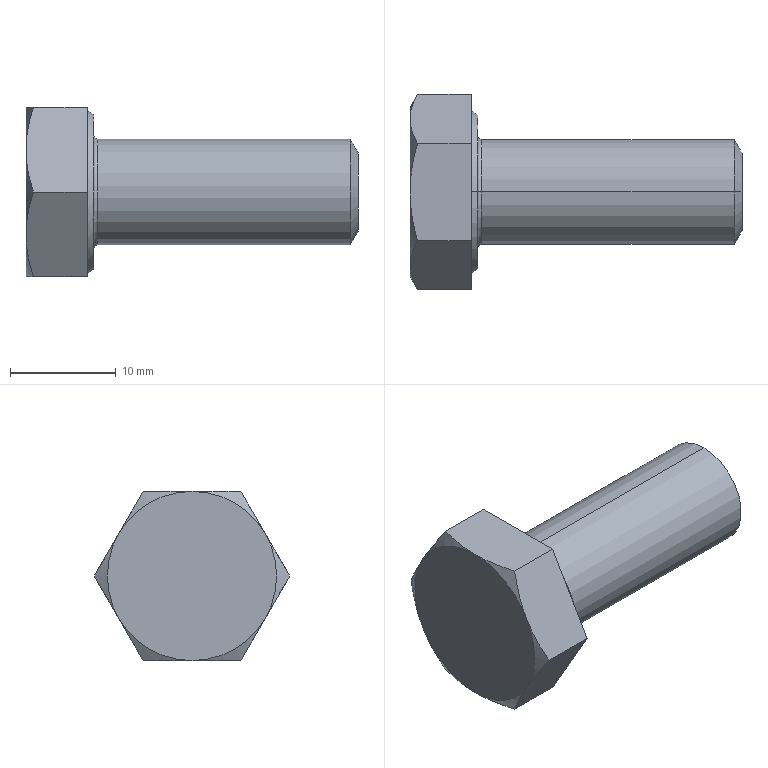Part | SolidWorks | features RevCut 3, Extrusion 1, Fillet 1, LPattern 1, Revolution 1 | 1 solid | 24 faces | box 31.4 x 18.475 x 16 mm | volume 3338 mm3 | cone 10 | plane 10 | torus 2 | cylinder 2 | commonest cylinder face diameters 10 x2
STEP:
#1=CARTESIAN_POINT('',(31.4,0.,3.701));
#2=VERTEX_POINT('',#1);
#3=CARTESIAN_POINT('',(31.4,0.,-3.701));
#4=VERTEX_POINT('',#3);
#5=CARTESIAN_POINT('',(31.4,0.,0.));
#6=DIRECTION('',(-1.,0.,0.));
#7=DIRECTION('',(0.,0.,1.));
#8=AXIS2_PLACEMENT_3D('',#5,#6,#7);
#9=CIRCLE('',#8,3.701);
#10=EDGE_CURVE('',#2,#4,#9,.T.);
#11=ORIENTED_EDGE('',*,*,#10,.T.);
#12=CARTESIAN_POINT('',(30.65,0.,-5.));
#13=VERTEX_POINT('',#12);
#14=CARTESIAN_POINT('',(30.65,0.,-5.));
#15=DIRECTION('',(-0.5,0.,-0.866));
#16=VECTOR('',#15,1000.);
#17=LINE('',#14,#16);
#18=EDGE_CURVE('',#4,#13,#17,.T.);
#19=ORIENTED_EDGE('',*,*,#18,.T.);
#20=CARTESIAN_POINT('',(30.65,0.,5.));
#21=VERTEX_POINT('',#20);
#22=CARTESIAN_POINT('',(30.65,0.,0.));
#23=DIRECTION('',(-1.,0.,0.));
#24=DIRECTION('',(0.,0.,1.));
#25=AXIS2_PLACEMENT_3D('',#22,#23,#24);
#26=CIRCLE('',#25,5.);
#27=EDGE_CURVE('',#21,#13,#26,.T.);
#28=ORIENTED_EDGE('',*,*,#27,.F.);
#29=CARTESIAN_POINT('',(30.65,0.,5.));
#30=DIRECTION('',(-0.5,0.,0.866));
#31=VECTOR('',#30,1000.);
#32=LINE('',#29,#31);
#33=EDGE_CURVE('',#2,#21,#32,.T.);
#34=ORIENTED_EDGE('',*,*,#33,.F.);
#35=EDGE_LOOP('',(#11,#19,#28,#34));
#36=FACE_OUTER_BOUND('',#35,.T.);
#37=CARTESIAN_POINT('',(30.65,0.,0.));
#38=DIRECTION('',(-1.,0.,0.));
#39=DIRECTION('',(0.,0.,1.));
#40=AXIS2_PLACEMENT_3D('',#37,#38,#39);
#41=CONICAL_SURFACE('',#40,5.,1.047);
#42=ADVANCED_FACE('',(#36),#41,.T.);
#43=CARTESIAN_POINT('',(6.8,0.,5.));
#44=VERTEX_POINT('',#43);
#45=CARTESIAN_POINT('',(6.8,0.,-5.));
#46=VERTEX_POINT('',#45);
#47=CARTESIAN_POINT('',(6.8,0.,0.));
#48=DIRECTION('',(1.,0.,0.));
#49=DIRECTION('',(0.,0.,-1.));
#50=AXIS2_PLACEMENT_3D('',#47,#48,#49);
#51=CIRCLE('',#50,5.);
#52=EDGE_CURVE('',#44,#46,#51,.T.);
#53=ORIENTED_EDGE('',*,*,#52,.F.);
#54=CARTESIAN_POINT('',(6.4,0.,5.4));
#55=VERTEX_POINT('',#54);
#56=CARTESIAN_POINT('',(6.8,0.,5.4));
#57=DIRECTION('',(0.,1.,0.));
#58=DIRECTION('',(0.,0.,1.));
#59=AXIS2_PLACEMENT_3D('',#56,#57,#58);
#60=CIRCLE('',#59,0.4);
#61=EDGE_CURVE('',#44,#55,#60,.T.);
#62=ORIENTED_EDGE('',*,*,#61,.T.);
#63=CARTESIAN_POINT('',(6.4,0.,-5.4));
#64=VERTEX_POINT('',#63);
#65=CARTESIAN_POINT('',(6.4,0.,0.));
#66=DIRECTION('',(-1.,0.,0.));
#67=DIRECTION('',(0.,0.,-1.));
#68=AXIS2_PLACEMENT_3D('',#65,#66,#67);
#69=CIRCLE('',#68,5.4);
#70=EDGE_CURVE('',#64,#55,#69,.T.);
#71=ORIENTED_EDGE('',*,*,#70,.F.);
#72=CARTESIAN_POINT('',(6.8,0.,-5.4));
#73=DIRECTION('',(0.,-1.,0.));
#74=DIRECTION('',(0.,0.,-1.));
#75=AXIS2_PLACEMENT_3D('',#72,#73,#74);
#76=CIRCLE('',#75,0.4);
#77=EDGE_CURVE('',#46,#64,#76,.T.);
#78=ORIENTED_EDGE('',*,*,#77,.F.);
#79=EDGE_LOOP('',(#53,#62,#71,#78));
#80=FACE_OUTER_BOUND('',#79,.T.);
#81=CARTESIAN_POINT('',(6.8,0.,0.));
#82=DIRECTION('',(1.,0.,0.));
#83=DIRECTION('',(0.,0.,-1.));
#84=AXIS2_PLACEMENT_3D('',#81,#82,#83);
#85=TOROIDAL_SURFACE('',#84,5.4,0.4);
#86=ADVANCED_FACE('',(#80),#85,.F.);
#87=CARTESIAN_POINT('',(6.4,0.,7.315));
#88=VERTEX_POINT('',#87);
#89=CARTESIAN_POINT('',(6.4,0.,-7.315));
#90=VERTEX_POINT('',#89);
#91=CARTESIAN_POINT('',(6.4,0.,0.));
#92=DIRECTION('',(-1.,0.,0.));
#93=DIRECTION('',(0.,0.,1.));
#94=AXIS2_PLACEMENT_3D('',#91,#92,#93);
#95=CIRCLE('',#94,7.315);
#96=EDGE_CURVE('',#88,#90,#95,.T.);
#97=ORIENTED_EDGE('',*,*,#96,.T.);
#98=CARTESIAN_POINT('',(5.8,0.,-7.661));
#99=VERTEX_POINT('',#98);
#100=CARTESIAN_POINT('',(5.8,0.,-7.661));
#101=DIRECTION('',(-0.866,0.,-0.5));
#102=VECTOR('',#101,1000.);
#103=LINE('',#100,#102);
#104=EDGE_CURVE('',#90,#99,#103,.T.);
#105=ORIENTED_EDGE('',*,*,#104,.T.);
#106=CARTESIAN_POINT('',(5.8,0.,7.661));
#107=VERTEX_POINT('',#106);
#108=CARTESIAN_POINT('',(5.8,0.,0.));
#109=DIRECTION('',(-1.,0.,0.));
#110=DIRECTION('',(0.,0.,1.));
#111=AXIS2_PLACEMENT_3D('',#108,#109,#110);
#112=CIRCLE('',#111,7.661);
#113=EDGE_CURVE('',#107,#99,#112,.T.);
#114=ORIENTED_EDGE('',*,*,#113,.F.);
#115=CARTESIAN_POINT('',(5.8,0.,7.661));
#116=DIRECTION('',(-0.866,0.,0.5));
#117=VECTOR('',#116,1000.);
#118=LINE('',#115,#117);
#119=EDGE_CURVE('',#88,#107,#118,.T.);
#120=ORIENTED_EDGE('',*,*,#119,.F.);
#121=EDGE_LOOP('',(#97,#105,#114,#120));
#122=FACE_OUTER_BOUND('',#121,.T.);
#123=CARTESIAN_POINT('',(5.8,0.,0.));
#124=DIRECTION('',(-1.,0.,0.));
#125=DIRECTION('',(0.,0.,1.));
#126=AXIS2_PLACEMENT_3D('',#123,#124,#125);
#127=CONICAL_SURFACE('',#126,7.661,0.5236);
#128=ADVANCED_FACE('',(#122),#127,.T.);
#129=ORIENTED_EDGE('',*,*,#27,.T.);
#130=CARTESIAN_POINT('',(0.,0.,-5.));
#131=DIRECTION('',(-1.,0.,0.));
#132=VECTOR('',#131,1000.);
#133=LINE('',#130,#132);
#134=EDGE_CURVE('',#13,#46,#133,.T.);
#135=ORIENTED_EDGE('',*,*,#134,.T.);
#136=CARTESIAN_POINT('',(6.8,0.,0.));
#137=DIRECTION('',(1.,0.,0.));
#138=DIRECTION('',(0.,0.,-1.));
#139=AXIS2_PLACEMENT_3D('',#136,#137,#138);
#140=CIRCLE('',#139,5.);
#141=EDGE_CURVE('',#46,#44,#140,.T.);
#142=ORIENTED_EDGE('',*,*,#141,.T.);
#143=CARTESIAN_POINT('',(0.,0.,5.));
#144=DIRECTION('',(-1.,0.,0.));
#145=VECTOR('',#144,1000.);
#146=LINE('',#143,#145);
#147=EDGE_CURVE('',#21,#44,#146,.T.);
#148=ORIENTED_EDGE('',*,*,#147,.F.);
#149=EDGE_LOOP('',(#129,#135,#142,#148));
#150=FACE_OUTER_BOUND('',#149,.T.);
#151=CARTESIAN_POINT('',(0.,0.,0.));
#152=DIRECTION('',(-1.,0.,0.));
#153=DIRECTION('',(0.,0.,1.));
#154=AXIS2_PLACEMENT_3D('',#151,#152,#153);
#155=CYLINDRICAL_SURFACE('',#154,5.);
#156=ADVANCED_FACE('',(#150),#155,.T.);
#157=ORIENTED_EDGE('',*,*,#134,.F.);
#158=CARTESIAN_POINT('',(30.65,0.,0.));
#159=DIRECTION('',(-1.,0.,0.));
#160=DIRECTION('',(0.,0.,1.));
#161=AXIS2_PLACEMENT_3D('',#158,#159,#160);
#162=CIRCLE('',#161,5.);
#163=EDGE_CURVE('',#13,#21,#162,.T.);
#164=ORIENTED_EDGE('',*,*,#163,.T.);
#165=ORIENTED_EDGE('',*,*,#147,.T.);
#166=ORIENTED_EDGE('',*,*,#52,.T.);
#167=EDGE_LOOP('',(#157,#164,#165,#166));
#168=FACE_OUTER_BOUND('',#167,.T.);
#169=CARTESIAN_POINT('',(0.,0.,0.));
#170=DIRECTION('',(-1.,0.,0.));
#171=DIRECTION('',(0.,0.,1.));
#172=AXIS2_PLACEMENT_3D('',#169,#170,#171);
#173=CYLINDRICAL_SURFACE('',#172,5.);
#174=ADVANCED_FACE('',(#168),#173,.T.);
#175=CARTESIAN_POINT('',(5.8,4.619,-8.));
#176=VERTEX_POINT('',#175);
#177=CARTESIAN_POINT('',(5.8,9.238,0.));
#178=VERTEX_POINT('',#177);
#179=CARTESIAN_POINT('',(5.8,4.619,-8.));
#180=DIRECTION('',(0.,0.5,0.866));
#181=VECTOR('',#180,1000.);
#182=LINE('',#179,#181);
#183=EDGE_CURVE('',#176,#178,#182,.T.);
#184=ORIENTED_EDGE('',*,*,#183,.F.);
#185=CARTESIAN_POINT('',(0.7145,4.619,-8.));
#186=VERTEX_POINT('',#185);
#187=CARTESIAN_POINT('',(6.4,4.619,-8.));
#188=DIRECTION('',(-1.,0.,0.));
#189=VECTOR('',#188,1000.);
#190=LINE('',#187,#189);
#191=EDGE_CURVE('',#176,#186,#190,.T.);
#192=ORIENTED_EDGE('',*,*,#191,.T.);
#193=CARTESIAN_POINT('',(0.,6.928,-4.));
#194=VERTEX_POINT('',#193);
#195=CARTESIAN_POINT('',(0.,6.928,-4.));
#196=CARTESIAN_POINT('',(0.,6.732,-4.339));
#197=CARTESIAN_POINT('',(0.01689,6.535,-4.68));
#198=CARTESIAN_POINT('',(0.08225,6.146,-5.355));
#199=CARTESIAN_POINT('',(0.1307,5.952,-5.69));
#200=CARTESIAN_POINT('',(0.3174,5.376,-6.689));
#201=CARTESIAN_POINT('',(0.497,4.996,-7.347));
#202=CARTESIAN_POINT('',(0.7145,4.619,-8.));
#203=B_SPLINE_CURVE_WITH_KNOTS('',3,(#195,#196,#197,#198,#199,#200,#201,#202),.UNSPECIFIED.,.F.,.F.,(4,2,2,4),(0.004674,0.005838,0.007002,0.00933),.UNSPECIFIED.);
#204=EDGE_CURVE('',#194,#186,#203,.T.);
#205=ORIENTED_EDGE('',*,*,#204,.F.);
#206=CARTESIAN_POINT('',(0.7145,9.238,0.));
#207=VERTEX_POINT('',#206);
#208=CARTESIAN_POINT('',(0.7145,9.238,0.));
#209=CARTESIAN_POINT('',(0.4964,8.86,-0.6543));
#210=CARTESIAN_POINT('',(0.3167,8.479,-1.313));
#211=CARTESIAN_POINT('',(0.0681,7.71,-2.646));
#212=CARTESIAN_POINT('',(0.,7.322,-3.319));
#213=CARTESIAN_POINT('',(0.,6.928,-4.));
#214=B_SPLINE_CURVE_WITH_KNOTS('',3,(#208,#209,#210,#211,#212,#213),.UNSPECIFIED.,.F.,.F.,(4,2,4),(0.000000238,0.002337,0.004674),.UNSPECIFIED.);
#215=EDGE_CURVE('',#207,#194,#214,.T.);
#216=ORIENTED_EDGE('',*,*,#215,.F.);
#217=CARTESIAN_POINT('',(6.4,9.238,0.));
#218=DIRECTION('',(-1.,0.,0.));
#219=VECTOR('',#218,1000.);
#220=LINE('',#217,#219);
#221=EDGE_CURVE('',#178,#207,#220,.T.);
#222=ORIENTED_EDGE('',*,*,#221,.F.);
#223=EDGE_LOOP('',(#184,#192,#205,#216,#222));
#224=FACE_OUTER_BOUND('',#223,.T.);
#225=CARTESIAN_POINT('',(6.4,4.619,-8.));
#226=DIRECTION('',(0.,-0.866,0.5));
#227=DIRECTION('',(0.,-0.5,-0.866));
#228=AXIS2_PLACEMENT_3D('',#225,#226,#227);
#229=PLANE('',#228);
#230=ADVANCED_FACE('',(#224),#229,.F.);
#231=CARTESIAN_POINT('',(5.8,4.619,8.));
#232=VERTEX_POINT('',#231);
#233=CARTESIAN_POINT('',(5.8,9.238,0.));
#234=DIRECTION('',(0.,-0.5,0.866));
#235=VECTOR('',#234,1000.);
#236=LINE('',#233,#235);
#237=EDGE_CURVE('',#178,#232,#236,.T.);
#238=ORIENTED_EDGE('',*,*,#237,.F.);
#239=ORIENTED_EDGE('',*,*,#221,.T.);
#240=CARTESIAN_POINT('',(0.,6.928,4.));
#241=VERTEX_POINT('',#240);
#242=CARTESIAN_POINT('',(0.,6.928,4.));
#243=CARTESIAN_POINT('',(0.,7.124,3.661));
#244=CARTESIAN_POINT('',(0.01689,7.321,3.32));
#245=CARTESIAN_POINT('',(0.08225,7.711,2.645));
#246=CARTESIAN_POINT('',(0.1307,7.904,2.31));
#247=CARTESIAN_POINT('',(0.3174,8.481,1.311));
#248=CARTESIAN_POINT('',(0.497,8.861,0.6527));
#249=CARTESIAN_POINT('',(0.7145,9.238,0.));
#250=B_SPLINE_CURVE_WITH_KNOTS('',3,(#242,#243,#244,#245,#246,#247,#248,#249),.UNSPECIFIED.,.F.,.F.,(4,2,2,4),(0.004674,0.005838,0.007002,0.00933),.UNSPECIFIED.);
#251=EDGE_CURVE('',#241,#207,#250,.T.);
#252=ORIENTED_EDGE('',*,*,#251,.F.);
#253=CARTESIAN_POINT('',(0.7145,4.619,8.));
#254=VERTEX_POINT('',#253);
#255=CARTESIAN_POINT('',(0.7145,4.619,8.));
#256=CARTESIAN_POINT('',(0.4964,4.997,7.346));
#257=CARTESIAN_POINT('',(0.3167,5.377,6.687));
#258=CARTESIAN_POINT('',(0.0681,6.146,5.354));
#259=CARTESIAN_POINT('',(0.,6.535,4.681));
#260=CARTESIAN_POINT('',(0.,6.928,4.));
#261=B_SPLINE_CURVE_WITH_KNOTS('',3,(#255,#256,#257,#258,#259,#260),.UNSPECIFIED.,.F.,.F.,(4,2,4),(0.000000238,0.002337,0.004674),.UNSPECIFIED.);
#262=EDGE_CURVE('',#254,#241,#261,.T.);
#263=ORIENTED_EDGE('',*,*,#262,.F.);
#264=CARTESIAN_POINT('',(6.4,4.619,8.));
#265=DIRECTION('',(-1.,0.,0.));
#266=VECTOR('',#265,1000.);
#267=LINE('',#264,#266);
#268=EDGE_CURVE('',#232,#254,#267,.T.);
#269=ORIENTED_EDGE('',*,*,#268,.F.);
#270=EDGE_LOOP('',(#238,#239,#252,#263,#269));
#271=FACE_OUTER_BOUND('',#270,.T.);
#272=CARTESIAN_POINT('',(6.4,9.238,0.));
#273=DIRECTION('',(0.,-0.866,-0.5));
#274=DIRECTION('',(0.,0.5,-0.866));
#275=AXIS2_PLACEMENT_3D('',#272,#273,#274);
#276=PLANE('',#275);
#277=ADVANCED_FACE('',(#271),#276,.F.);
#278=CARTESIAN_POINT('',(5.8,-4.619,8.));
#279=VERTEX_POINT('',#278);
#280=CARTESIAN_POINT('',(5.8,4.619,8.));
#281=DIRECTION('',(0.,-1.,0.));
#282=VECTOR('',#281,1000.);
#283=LINE('',#280,#282);
#284=EDGE_CURVE('',#232,#279,#283,.T.);
#285=ORIENTED_EDGE('',*,*,#284,.F.);
#286=ORIENTED_EDGE('',*,*,#268,.T.);
#287=CARTESIAN_POINT('',(0.,0.,8.));
#288=VERTEX_POINT('',#287);
#289=CARTESIAN_POINT('',(0.,0.,8.));
#290=CARTESIAN_POINT('',(0.,0.3913,8.));
#291=CARTESIAN_POINT('',(0.01678,0.7854,8.));
#292=CARTESIAN_POINT('',(0.08286,1.571,8.));
#293=CARTESIAN_POINT('',(0.1318,1.96,8.));
#294=CARTESIAN_POINT('',(0.3194,3.115,8.));
#295=CARTESIAN_POINT('',(0.4988,3.872,8.));
#296=CARTESIAN_POINT('',(0.7145,4.619,8.));
#297=B_SPLINE_CURVE_WITH_KNOTS('',3,(#289,#290,#291,#292,#293,#294,#295,#296),.UNSPECIFIED.,.F.,.F.,(4,2,2,4),(0.01337,0.01454,0.01571,0.01805),.UNSPECIFIED.);
#298=EDGE_CURVE('',#288,#254,#297,.T.);
#299=ORIENTED_EDGE('',*,*,#298,.F.);
#300=CARTESIAN_POINT('',(0.7145,-4.619,8.));
#301=VERTEX_POINT('',#300);
#302=CARTESIAN_POINT('',(0.7145,-4.619,8.));
#303=CARTESIAN_POINT('',(0.4973,-3.866,8.));
#304=CARTESIAN_POINT('',(0.3158,-3.098,8.));
#305=CARTESIAN_POINT('',(0.0673,-1.557,8.));
#306=CARTESIAN_POINT('',(0.,-0.7819,8.));
#307=CARTESIAN_POINT('',(0.,0.,8.));
#308=B_SPLINE_CURVE_WITH_KNOTS('',3,(#302,#303,#304,#305,#306,#307),.UNSPECIFIED.,.F.,.F.,(4,2,4),(0.00869,0.01103,0.01337),.UNSPECIFIED.);
#309=EDGE_CURVE('',#301,#288,#308,.T.);
#310=ORIENTED_EDGE('',*,*,#309,.F.);
#311=CARTESIAN_POINT('',(6.4,-4.619,8.));
#312=DIRECTION('',(-1.,0.,0.));
#313=VECTOR('',#312,1000.);
#314=LINE('',#311,#313);
#315=EDGE_CURVE('',#279,#301,#314,.T.);
#316=ORIENTED_EDGE('',*,*,#315,.F.);
#317=EDGE_LOOP('',(#285,#286,#299,#310,#316));
#318=FACE_OUTER_BOUND('',#317,.T.);
#319=CARTESIAN_POINT('',(6.4,4.619,8.));
#320=DIRECTION('',(0.,0.,-1.));
#321=DIRECTION('',(-1.,0.,0.));
#322=AXIS2_PLACEMENT_3D('',#319,#320,#321);
#323=PLANE('',#322);
#324=ADVANCED_FACE('',(#318),#323,.F.);
#325=CARTESIAN_POINT('',(5.8,-9.238,0.));
#326=VERTEX_POINT('',#325);
#327=CARTESIAN_POINT('',(5.8,-9.238,0.));
#328=DIRECTION('',(0.,-0.5,-0.866));
#329=VECTOR('',#328,1000.);
#330=LINE('',#327,#329);
#331=EDGE_CURVE('',#279,#326,#330,.T.);
#332=ORIENTED_EDGE('',*,*,#331,.F.);
#333=ORIENTED_EDGE('',*,*,#315,.T.);
#334=CARTESIAN_POINT('',(0.,-6.928,4.));
#335=VERTEX_POINT('',#334);
#336=CARTESIAN_POINT('',(0.,-6.928,4.));
#337=CARTESIAN_POINT('',(0.,-6.732,4.339));
#338=CARTESIAN_POINT('',(0.01689,-6.535,4.68));
#339=CARTESIAN_POINT('',(0.08225,-6.146,5.355));
#340=CARTESIAN_POINT('',(0.1307,-5.952,5.69));
#341=CARTESIAN_POINT('',(0.3174,-5.376,6.689));
#342=CARTESIAN_POINT('',(0.497,-4.996,7.347));
#343=CARTESIAN_POINT('',(0.7145,-4.619,8.));
#344=B_SPLINE_CURVE_WITH_KNOTS('',3,(#336,#337,#338,#339,#340,#341,#342,#343),.UNSPECIFIED.,.F.,.F.,(4,2,2,4),(0.004674,0.005838,0.007002,0.00933),.UNSPECIFIED.);
#345=EDGE_CURVE('',#335,#301,#344,.T.);
#346=ORIENTED_EDGE('',*,*,#345,.F.);
#347=CARTESIAN_POINT('',(0.7145,-9.238,0.));
#348=VERTEX_POINT('',#347);
#349=CARTESIAN_POINT('',(0.7145,-9.238,0.));
#350=CARTESIAN_POINT('',(0.4964,-8.86,0.6543));
#351=CARTESIAN_POINT('',(0.3167,-8.479,1.313));
#352=CARTESIAN_POINT('',(0.0681,-7.71,2.646));
#353=CARTESIAN_POINT('',(0.,-7.322,3.319));
#354=CARTESIAN_POINT('',(0.,-6.928,4.));
#355=B_SPLINE_CURVE_WITH_KNOTS('',3,(#349,#350,#351,#352,#353,#354),.UNSPECIFIED.,.F.,.F.,(4,2,4),(0.000000238,0.002337,0.004674),.UNSPECIFIED.);
#356=EDGE_CURVE('',#348,#335,#355,.T.);
#357=ORIENTED_EDGE('',*,*,#356,.F.);
#358=CARTESIAN_POINT('',(6.4,-9.238,0.));
#359=DIRECTION('',(-1.,0.,0.));
#360=VECTOR('',#359,1000.);
#361=LINE('',#358,#360);
#362=EDGE_CURVE('',#326,#348,#361,.T.);
#363=ORIENTED_EDGE('',*,*,#362,.F.);
#364=EDGE_LOOP('',(#332,#333,#346,#357,#363));
#365=FACE_OUTER_BOUND('',#364,.T.);
#366=CARTESIAN_POINT('',(6.4,-9.238,0.));
#367=DIRECTION('',(0.,0.866,-0.5));
#368=DIRECTION('',(0.,0.5,0.866));
#369=AXIS2_PLACEMENT_3D('',#366,#367,#368);
#370=PLANE('',#369);
#371=ADVANCED_FACE('',(#365),#370,.F.);
#372=CARTESIAN_POINT('',(5.8,-4.619,-8.));
#373=VERTEX_POINT('',#372);
#374=CARTESIAN_POINT('',(5.8,-4.619,-8.));
#375=DIRECTION('',(0.,0.5,-0.866));
#376=VECTOR('',#375,1000.);
#377=LINE('',#374,#376);
#378=EDGE_CURVE('',#326,#373,#377,.T.);
#379=ORIENTED_EDGE('',*,*,#378,.F.);
#380=ORIENTED_EDGE('',*,*,#362,.T.);
#381=CARTESIAN_POINT('',(0.,-6.928,-4.));
#382=VERTEX_POINT('',#381);
#383=CARTESIAN_POINT('',(0.,-6.928,-4.));
#384=CARTESIAN_POINT('',(0.,-7.124,-3.661));
#385=CARTESIAN_POINT('',(0.01689,-7.321,-3.32));
#386=CARTESIAN_POINT('',(0.08225,-7.711,-2.645));
#387=CARTESIAN_POINT('',(0.1307,-7.904,-2.31));
#388=CARTESIAN_POINT('',(0.3174,-8.481,-1.311));
#389=CARTESIAN_POINT('',(0.497,-8.861,-0.6527));
#390=CARTESIAN_POINT('',(0.7145,-9.238,0.));
#391=B_SPLINE_CURVE_WITH_KNOTS('',3,(#383,#384,#385,#386,#387,#388,#389,#390),.UNSPECIFIED.,.F.,.F.,(4,2,2,4),(0.004674,0.005838,0.007002,0.00933),.UNSPECIFIED.);
#392=EDGE_CURVE('',#382,#348,#391,.T.);
#393=ORIENTED_EDGE('',*,*,#392,.F.);
#394=CARTESIAN_POINT('',(0.7145,-4.619,-8.));
#395=VERTEX_POINT('',#394);
#396=CARTESIAN_POINT('',(0.7145,-4.619,-8.));
#397=CARTESIAN_POINT('',(0.4964,-4.997,-7.346));
#398=CARTESIAN_POINT('',(0.3167,-5.377,-6.687));
#399=CARTESIAN_POINT('',(0.0681,-6.146,-5.354));
#400=CARTESIAN_POINT('',(0.,-6.535,-4.681));
#401=CARTESIAN_POINT('',(0.,-6.928,-4.));
#402=B_SPLINE_CURVE_WITH_KNOTS('',3,(#396,#397,#398,#399,#400,#401),.UNSPECIFIED.,.F.,.F.,(4,2,4),(0.000000238,0.002337,0.004674),.UNSPECIFIED.);
#403=EDGE_CURVE('',#395,#382,#402,.T.);
#404=ORIENTED_EDGE('',*,*,#403,.F.);
#405=CARTESIAN_POINT('',(6.4,-4.619,-8.));
#406=DIRECTION('',(-1.,0.,0.));
#407=VECTOR('',#406,1000.);
#408=LINE('',#405,#407);
#409=EDGE_CURVE('',#373,#395,#408,.T.);
#410=ORIENTED_EDGE('',*,*,#409,.F.);
#411=EDGE_LOOP('',(#379,#380,#393,#404,#410));
#412=FACE_OUTER_BOUND('',#411,.T.);
#413=CARTESIAN_POINT('',(6.4,-4.619,-8.));
#414=DIRECTION('',(0.,0.866,0.5));
#415=DIRECTION('',(0.,-0.5,0.866));
#416=AXIS2_PLACEMENT_3D('',#413,#414,#415);
#417=PLANE('',#416);
#418=ADVANCED_FACE('',(#412),#417,.F.);
#419=CARTESIAN_POINT('',(5.8,4.619,-8.));
#420=DIRECTION('',(0.,1.,0.));
#421=VECTOR('',#420,1000.);
#422=LINE('',#419,#421);
#423=EDGE_CURVE('',#373,#176,#422,.T.);
#424=ORIENTED_EDGE('',*,*,#423,.F.);
#425=ORIENTED_EDGE('',*,*,#409,.T.);
#426=CARTESIAN_POINT('',(0.,0.,-8.));
#427=VERTEX_POINT('',#426);
#428=CARTESIAN_POINT('',(0.,0.,-8.));
#429=CARTESIAN_POINT('',(0.,-0.7819,-8.));
#430=CARTESIAN_POINT('',(0.0673,-1.557,-8.));
#431=CARTESIAN_POINT('',(0.3158,-3.098,-8.));
#432=CARTESIAN_POINT('',(0.4973,-3.866,-8.));
#433=CARTESIAN_POINT('',(0.7145,-4.619,-8.));
#434=B_SPLINE_CURVE_WITH_KNOTS('',3,(#428,#429,#430,#431,#432,#433),.UNSPECIFIED.,.F.,.F.,(4,2,4),(0.02753,0.02987,0.03221),.UNSPECIFIED.);
#435=EDGE_CURVE('',#427,#395,#434,.T.);
#436=ORIENTED_EDGE('',*,*,#435,.F.);
#437=CARTESIAN_POINT('',(0.7145,4.619,-8.));
#438=CARTESIAN_POINT('',(0.4988,3.872,-8.));
#439=CARTESIAN_POINT('',(0.3194,3.115,-8.));
#440=CARTESIAN_POINT('',(0.1318,1.96,-8.));
#441=CARTESIAN_POINT('',(0.08286,1.571,-8.));
#442=CARTESIAN_POINT('',(0.01678,0.7854,-8.));
#443=CARTESIAN_POINT('',(0.,0.3913,-8.));
#444=CARTESIAN_POINT('',(0.,0.,-8.));
#445=B_SPLINE_CURVE_WITH_KNOTS('',3,(#437,#438,#439,#440,#441,#442,#443,#444),.UNSPECIFIED.,.F.,.F.,(4,2,2,4),(0.02285,0.02519,0.02636,0.02753),.UNSPECIFIED.);
#446=EDGE_CURVE('',#186,#427,#445,.T.);
#447=ORIENTED_EDGE('',*,*,#446,.F.);
#448=ORIENTED_EDGE('',*,*,#191,.F.);
#449=EDGE_LOOP('',(#424,#425,#436,#447,#448));
#450=FACE_OUTER_BOUND('',#449,.T.);
#451=CARTESIAN_POINT('',(6.4,4.619,-8.));
#452=DIRECTION('',(0.,0.,1.));
#453=DIRECTION('',(0.,-1.,0.));
#454=AXIS2_PLACEMENT_3D('',#451,#452,#453);
#455=PLANE('',#454);
#456=ADVANCED_FACE('',(#450),#455,.F.);
#457=ORIENTED_EDGE('',*,*,#403,.T.);
#458=CARTESIAN_POINT('',(0.,0.,0.));
#459=DIRECTION('',(1.,0.,0.));
#460=DIRECTION('',(0.,0.,-1.));
#461=AXIS2_PLACEMENT_3D('',#458,#459,#460);
#462=CIRCLE('',#461,8.);
#463=EDGE_CURVE('',#382,#427,#462,.T.);
#464=ORIENTED_EDGE('',*,*,#463,.T.);
#465=ORIENTED_EDGE('',*,*,#435,.T.);
#466=EDGE_LOOP('',(#457,#464,#465));
#467=FACE_OUTER_BOUND('',#466,.T.);
#468=CARTESIAN_POINT('',(0.,0.,0.));
#469=DIRECTION('',(1.,0.,0.));
#470=DIRECTION('',(0.,0.,-1.));
#471=AXIS2_PLACEMENT_3D('',#468,#469,#470);
#472=CONICAL_SURFACE('',#471,8.,1.047);
#473=ADVANCED_FACE('',(#467),#472,.T.);
#474=ORIENTED_EDGE('',*,*,#356,.T.);
#475=CARTESIAN_POINT('',(0.,0.,0.));
#476=DIRECTION('',(1.,0.,0.));
#477=DIRECTION('',(0.,0.,-1.));
#478=AXIS2_PLACEMENT_3D('',#475,#476,#477);
#479=CIRCLE('',#478,8.);
#480=EDGE_CURVE('',#335,#382,#479,.T.);
#481=ORIENTED_EDGE('',*,*,#480,.T.);
#482=ORIENTED_EDGE('',*,*,#392,.T.);
#483=EDGE_LOOP('',(#474,#481,#482));
#484=FACE_OUTER_BOUND('',#483,.T.);
#485=CARTESIAN_POINT('',(0.,0.,0.));
#486=DIRECTION('',(1.,0.,0.));
#487=DIRECTION('',(0.,0.,-1.));
#488=AXIS2_PLACEMENT_3D('',#485,#486,#487);
#489=CONICAL_SURFACE('',#488,8.,1.047);
#490=ADVANCED_FACE('',(#484),#489,.T.);
#491=ORIENTED_EDGE('',*,*,#309,.T.);
#492=CARTESIAN_POINT('',(0.,0.,0.));
#493=DIRECTION('',(1.,0.,0.));
#494=DIRECTION('',(0.,0.,-1.));
#495=AXIS2_PLACEMENT_3D('',#492,#493,#494);
#496=CIRCLE('',#495,8.);
#497=EDGE_CURVE('',#288,#335,#496,.T.);
#498=ORIENTED_EDGE('',*,*,#497,.T.);
#499=ORIENTED_EDGE('',*,*,#345,.T.);
#500=EDGE_LOOP('',(#491,#498,#499));
#501=FACE_OUTER_BOUND('',#500,.T.);
#502=CARTESIAN_POINT('',(0.,0.,0.));
#503=DIRECTION('',(1.,0.,0.));
#504=DIRECTION('',(0.,0.,-1.));
#505=AXIS2_PLACEMENT_3D('',#502,#503,#504);
#506=CONICAL_SURFACE('',#505,8.,1.047);
#507=ADVANCED_FACE('',(#501),#506,.T.);
#508=ORIENTED_EDGE('',*,*,#298,.T.);
#509=ORIENTED_EDGE('',*,*,#262,.T.);
#510=CARTESIAN_POINT('',(0.,0.,0.));
#511=DIRECTION('',(-1.,0.,0.));
#512=DIRECTION('',(0.,0.,1.));
#513=AXIS2_PLACEMENT_3D('',#510,#511,#512);
#514=CIRCLE('',#513,8.);
#515=EDGE_CURVE('',#288,#241,#514,.T.);
#516=ORIENTED_EDGE('',*,*,#515,.F.);
#517=EDGE_LOOP('',(#508,#509,#516));
#518=FACE_OUTER_BOUND('',#517,.T.);
#519=CARTESIAN_POINT('',(0.,0.,0.));
#520=DIRECTION('',(1.,0.,0.));
#521=DIRECTION('',(0.,0.,-1.));
#522=AXIS2_PLACEMENT_3D('',#519,#520,#521);
#523=CONICAL_SURFACE('',#522,8.,1.047);
#524=ADVANCED_FACE('',(#518),#523,.T.);
#525=ORIENTED_EDGE('',*,*,#251,.T.);
#526=ORIENTED_EDGE('',*,*,#215,.T.);
#527=CARTESIAN_POINT('',(0.,0.,0.));
#528=DIRECTION('',(1.,0.,0.));
#529=DIRECTION('',(0.,0.,-1.));
#530=AXIS2_PLACEMENT_3D('',#527,#528,#529);
#531=CIRCLE('',#530,8.);
#532=EDGE_CURVE('',#194,#241,#531,.T.);
#533=ORIENTED_EDGE('',*,*,#532,.T.);
#534=EDGE_LOOP('',(#525,#526,#533));
#535=FACE_OUTER_BOUND('',#534,.T.);
#536=CARTESIAN_POINT('',(0.,0.,0.));
#537=DIRECTION('',(1.,0.,0.));
#538=DIRECTION('',(0.,0.,-1.));
#539=AXIS2_PLACEMENT_3D('',#536,#537,#538);
#540=CONICAL_SURFACE('',#539,8.,1.047);
#541=ADVANCED_FACE('',(#535),#540,.T.);
#542=ORIENTED_EDGE('',*,*,#204,.T.);
#543=ORIENTED_EDGE('',*,*,#446,.T.);
#544=CARTESIAN_POINT('',(0.,0.,0.));
#545=DIRECTION('',(1.,0.,0.));
#546=DIRECTION('',(0.,0.,-1.));
#547=AXIS2_PLACEMENT_3D('',#544,#545,#546);
#548=CIRCLE('',#547,8.);
#549=EDGE_CURVE('',#427,#194,#548,.T.);
#550=ORIENTED_EDGE('',*,*,#549,.T.);
#551=EDGE_LOOP('',(#542,#543,#550));
#552=FACE_OUTER_BOUND('',#551,.T.);
#553=CARTESIAN_POINT('',(0.,0.,0.));
#554=DIRECTION('',(1.,0.,0.));
#555=DIRECTION('',(0.,0.,-1.));
#556=AXIS2_PLACEMENT_3D('',#553,#554,#555);
#557=CONICAL_SURFACE('',#556,8.,1.047);
#558=ADVANCED_FACE('',(#552),#557,.T.);
#559=ORIENTED_EDGE('',*,*,#549,.F.);
#560=ORIENTED_EDGE('',*,*,#463,.F.);
#561=ORIENTED_EDGE('',*,*,#480,.F.);
#562=ORIENTED_EDGE('',*,*,#497,.F.);
#563=ORIENTED_EDGE('',*,*,#515,.T.);
#564=ORIENTED_EDGE('',*,*,#532,.F.);
#565=EDGE_LOOP('',(#559,#560,#561,#562,#563,#564));
#566=FACE_OUTER_BOUND('',#565,.T.);
#567=CARTESIAN_POINT('',(0.,0.,-16.));
#568=DIRECTION('',(1.,0.,0.));
#569=DIRECTION('',(0.,0.,-1.));
#570=AXIS2_PLACEMENT_3D('',#567,#568,#569);
#571=PLANE('',#570);
#572=ADVANCED_FACE('',(#566),#571,.F.);
#573=ORIENTED_EDGE('',*,*,#113,.T.);
#574=CARTESIAN_POINT('',(5.8,0.,0.));
#575=DIRECTION('',(-1.,0.,0.));
#576=DIRECTION('',(0.,0.,1.));
#577=AXIS2_PLACEMENT_3D('',#574,#575,#576);
#578=CIRCLE('',#577,7.661);
#579=EDGE_CURVE('',#99,#107,#578,.T.);
#580=ORIENTED_EDGE('',*,*,#579,.T.);
#581=EDGE_LOOP('',(#573,#580));
#582=FACE_BOUND('',#581,.T.);
#583=ORIENTED_EDGE('',*,*,#183,.T.);
#584=ORIENTED_EDGE('',*,*,#237,.T.);
#585=ORIENTED_EDGE('',*,*,#284,.T.);
#586=ORIENTED_EDGE('',*,*,#331,.T.);
#587=ORIENTED_EDGE('',*,*,#378,.T.);
#588=ORIENTED_EDGE('',*,*,#423,.T.);
#589=EDGE_LOOP('',(#583,#584,#585,#586,#587,#588));
#590=FACE_OUTER_BOUND('',#589,.T.);
#591=CARTESIAN_POINT('',(5.8,7.661,0.));
#592=DIRECTION('',(1.,0.,0.));
#593=DIRECTION('',(0.,0.,-1.));
#594=AXIS2_PLACEMENT_3D('',#591,#592,#593);
#595=PLANE('',#594);
#596=ADVANCED_FACE('',(#582,#590),#595,.T.);
#597=ORIENTED_EDGE('',*,*,#104,.F.);
#598=CARTESIAN_POINT('',(6.4,0.,0.));
#599=DIRECTION('',(-1.,0.,0.));
#600=DIRECTION('',(0.,0.,1.));
#601=AXIS2_PLACEMENT_3D('',#598,#599,#600);
#602=CIRCLE('',#601,7.315);
#603=EDGE_CURVE('',#90,#88,#602,.T.);
#604=ORIENTED_EDGE('',*,*,#603,.T.);
#605=ORIENTED_EDGE('',*,*,#119,.T.);
#606=ORIENTED_EDGE('',*,*,#579,.F.);
#607=EDGE_LOOP('',(#597,#604,#605,#606));
#608=FACE_OUTER_BOUND('',#607,.T.);
#609=CARTESIAN_POINT('',(5.8,0.,0.));
#610=DIRECTION('',(-1.,0.,0.));
#611=DIRECTION('',(0.,0.,1.));
#612=AXIS2_PLACEMENT_3D('',#609,#610,#611);
#613=CONICAL_SURFACE('',#612,7.661,0.5236);
#614=ADVANCED_FACE('',(#608),#613,.T.);
#615=ORIENTED_EDGE('',*,*,#70,.T.);
#616=CARTESIAN_POINT('',(6.4,0.,0.));
#617=DIRECTION('',(-1.,0.,0.));
#618=DIRECTION('',(0.,0.,-1.));
#619=AXIS2_PLACEMENT_3D('',#616,#617,#618);
#620=CIRCLE('',#619,5.4);
#621=EDGE_CURVE('',#55,#64,#620,.T.);
#622=ORIENTED_EDGE('',*,*,#621,.T.);
#623=EDGE_LOOP('',(#615,#622));
#624=FACE_BOUND('',#623,.T.);
#625=ORIENTED_EDGE('',*,*,#96,.F.);
#626=ORIENTED_EDGE('',*,*,#603,.F.);
#627=EDGE_LOOP('',(#625,#626));
#628=FACE_OUTER_BOUND('',#627,.T.);
#629=CARTESIAN_POINT('',(6.4,0.,-16.));
#630=DIRECTION('',(1.,0.,0.));
#631=DIRECTION('',(0.,0.,-1.));
#632=AXIS2_PLACEMENT_3D('',#629,#630,#631);
#633=PLANE('',#632);
#634=ADVANCED_FACE('',(#624,#628),#633,.T.);
#635=ORIENTED_EDGE('',*,*,#61,.F.);
#636=ORIENTED_EDGE('',*,*,#141,.F.);
#637=ORIENTED_EDGE('',*,*,#77,.T.);
#638=ORIENTED_EDGE('',*,*,#621,.F.);
#639=EDGE_LOOP('',(#635,#636,#637,#638));
#640=FACE_OUTER_BOUND('',#639,.T.);
#641=CARTESIAN_POINT('',(6.8,0.,0.));
#642=DIRECTION('',(1.,0.,0.));
#643=DIRECTION('',(0.,0.,-1.));
#644=AXIS2_PLACEMENT_3D('',#641,#642,#643);
#645=TOROIDAL_SURFACE('',#644,5.4,0.4);
#646=ADVANCED_FACE('',(#640),#645,.F.);
#647=ORIENTED_EDGE('',*,*,#18,.F.);
#648=CARTESIAN_POINT('',(31.4,0.,0.));
#649=DIRECTION('',(-1.,0.,0.));
#650=DIRECTION('',(0.,0.,1.));
#651=AXIS2_PLACEMENT_3D('',#648,#649,#650);
#652=CIRCLE('',#651,3.701);
#653=EDGE_CURVE('',#4,#2,#652,.T.);
#654=ORIENTED_EDGE('',*,*,#653,.T.);
#655=ORIENTED_EDGE('',*,*,#33,.T.);
#656=ORIENTED_EDGE('',*,*,#163,.F.);
#657=EDGE_LOOP('',(#647,#654,#655,#656));
#658=FACE_OUTER_BOUND('',#657,.T.);
#659=CARTESIAN_POINT('',(30.65,0.,0.));
#660=DIRECTION('',(-1.,0.,0.));
#661=DIRECTION('',(0.,0.,1.));
#662=AXIS2_PLACEMENT_3D('',#659,#660,#661);
#663=CONICAL_SURFACE('',#662,5.,1.047);
#664=ADVANCED_FACE('',(#658),#663,.T.);
#665=ORIENTED_EDGE('',*,*,#10,.F.);
#666=ORIENTED_EDGE('',*,*,#653,.F.);
#667=EDGE_LOOP('',(#665,#666));
#668=FACE_OUTER_BOUND('',#667,.T.);
#669=CARTESIAN_POINT('',(31.4,0.,0.));
#670=DIRECTION('',(-1.,0.,0.));
#671=DIRECTION('',(0.,0.,1.));
#672=AXIS2_PLACEMENT_3D('',#669,#670,#671);
#673=PLANE('',#672);
#674=ADVANCED_FACE('',(#668),#673,.F.);
#675=CLOSED_SHELL('',(#42,#86,#128,#156,#174,#230,#277,#324,#371,#418,#456,#473,#490,#507,#524,#541,#558,#572,#596,#614,#634,#646,#664,#674));
#676=MANIFOLD_SOLID_BREP('',#675);
#677=CARTESIAN_POINT('',(0.,0.,0.));
#678=DIRECTION('',(0.,0.,1.));
#679=DIRECTION('',(1.,0.,0.));
#680=AXIS2_PLACEMENT_3D('',#677,#678,#679);
#681=(LENGTH_UNIT()NAMED_UNIT(*)SI_UNIT(.MILLI.,.METRE.));
#682=UNCERTAINTY_MEASURE_WITH_UNIT(LENGTH_MEASURE(0.00001),#681,'','');
#683=(NAMED_UNIT(*)PLANE_ANGLE_UNIT()SI_UNIT($,.RADIAN.));
#684=(NAMED_UNIT(*)SI_UNIT($,.STERADIAN.)SOLID_ANGLE_UNIT());
#685=(GEOMETRIC_REPRESENTATION_CONTEXT(3)GLOBAL_UNCERTAINTY_ASSIGNED_CONTEXT((#682))GLOBAL_UNIT_ASSIGNED_CONTEXT((#681,#683,#684))REPRESENTATION_CONTEXT('',''));
#686=ADVANCED_BREP_SHAPE_REPRESENTATION('',(#676,#680),#685);